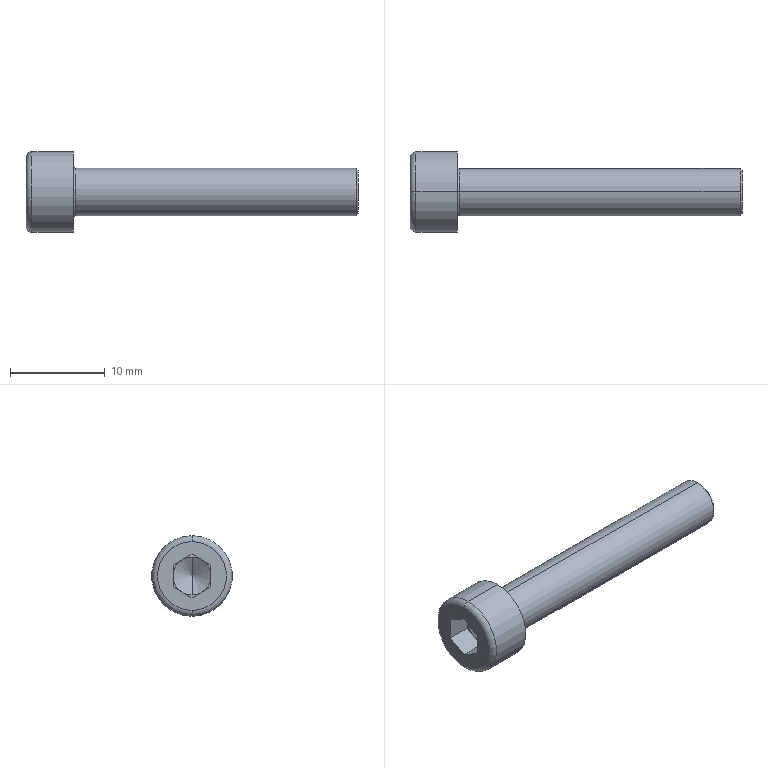Part | STEP file | GB_Hex socket head cylinder screw_M5X30_M5X30 | 1 solid | 27 faces | box 35 x 8.5 x 8.5 mm | volume 830.962 mm3 | plane 15 | cone 4 | torus 4 | cylinder 4 | commonest cylinder face diameters 5 x2 8.5 x2